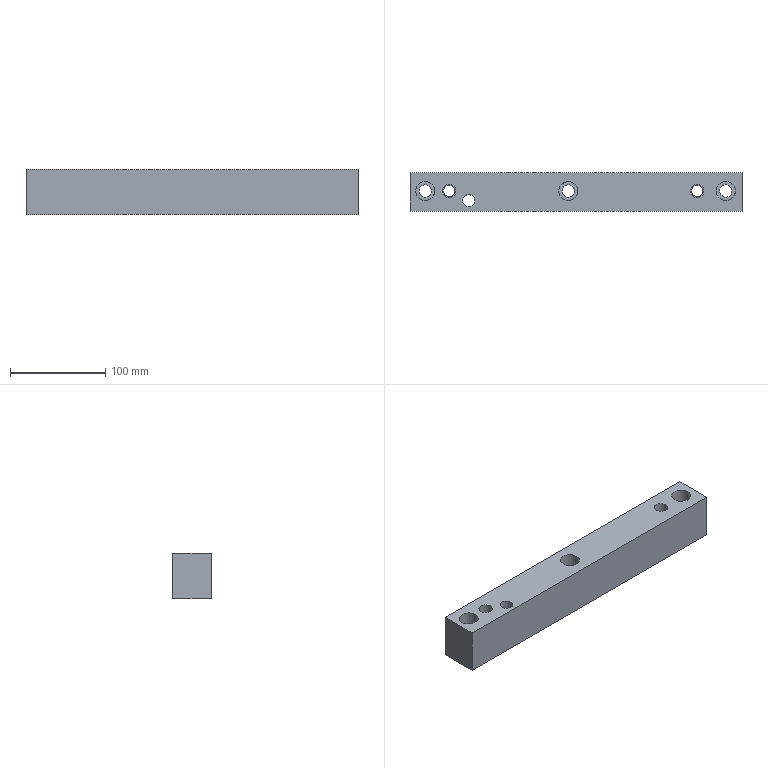Part | STEP file | gslz 2016.10.28-13_id1338_x_t | 1 solid | 22 faces | box 348 x 40 x 48 mm | volume 621204 mm3 | plane 11 | cylinder 11 | commonest cylinder face diameters 13 x4 20 x3 12 x2 14 x2